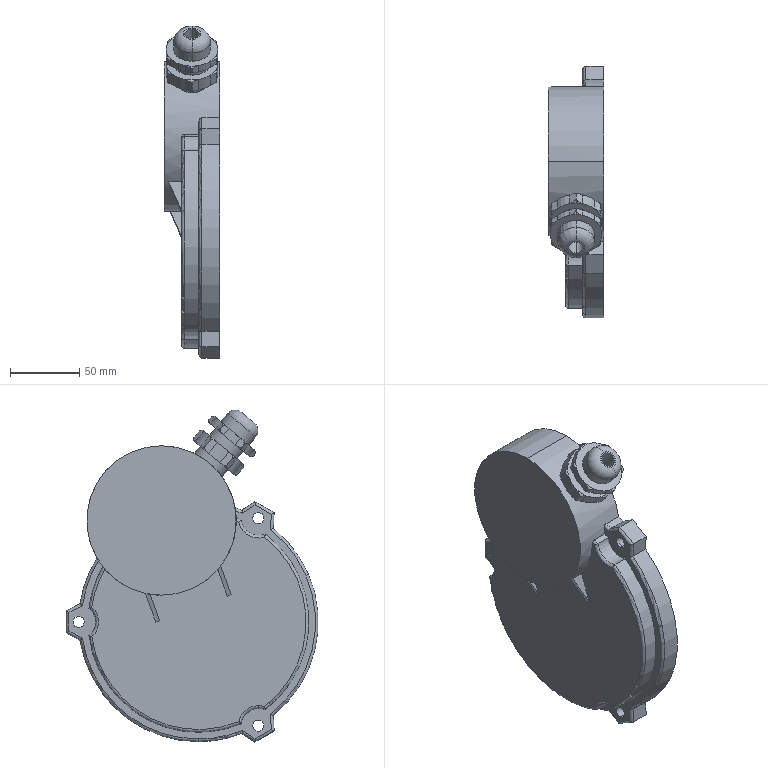Part | SolidWorks | features BaseBody 1 | 1 solid | 146 faces | box 39.9 x 182.18 x 239.915 mm | volume 603976 mm3 | cylinder 53 | plane 50 | torus 43 | commonest cylinder face diameters 37.4 x12 4 x9 8 x6 26.4 x6 159.5 x5 173.18 x5